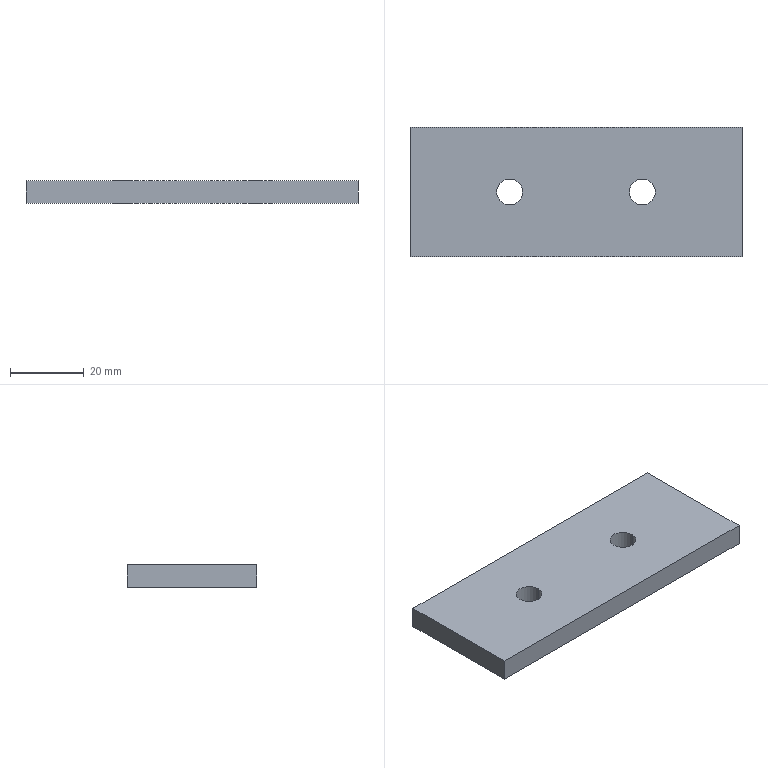Part | SolidWorks | features Extrusion 1, HoleWzd 1 | 1 solid | 10 faces | box 90 x 35 x 6 mm | volume 18438 mm3 | plane 6 | cylinder 4 | commonest cylinder face diameters 7 x4
STEP:
#1=CARTESIAN_POINT('',(23.5,17.5,0.));
#2=VERTEX_POINT('',#1);
#3=CARTESIAN_POINT('',(30.5,17.5,0.));
#4=VERTEX_POINT('',#3);
#5=CARTESIAN_POINT('',(27.,17.5,0.));
#6=DIRECTION('',(0.,0.,1.));
#7=DIRECTION('',(1.,0.,0.));
#8=AXIS2_PLACEMENT_3D('',#5,#6,#7);
#9=CIRCLE('',#8,3.5);
#10=EDGE_CURVE('',#2,#4,#9,.T.);
#11=ORIENTED_EDGE('',*,*,#10,.F.);
#12=CARTESIAN_POINT('',(23.5,17.5,6.));
#13=VERTEX_POINT('',#12);
#14=CARTESIAN_POINT('',(23.5,17.5,6.));
#15=DIRECTION('',(0.,0.,1.));
#16=VECTOR('',#15,1000.);
#17=LINE('',#14,#16);
#18=EDGE_CURVE('',#2,#13,#17,.T.);
#19=ORIENTED_EDGE('',*,*,#18,.T.);
#20=CARTESIAN_POINT('',(30.5,17.5,6.));
#21=VERTEX_POINT('',#20);
#22=CARTESIAN_POINT('',(27.,17.5,6.));
#23=DIRECTION('',(0.,0.,1.));
#24=DIRECTION('',(1.,0.,0.));
#25=AXIS2_PLACEMENT_3D('',#22,#23,#24);
#26=CIRCLE('',#25,3.5);
#27=EDGE_CURVE('',#13,#21,#26,.T.);
#28=ORIENTED_EDGE('',*,*,#27,.T.);
#29=CARTESIAN_POINT('',(30.5,17.5,6.));
#30=DIRECTION('',(0.,0.,1.));
#31=VECTOR('',#30,1000.);
#32=LINE('',#29,#31);
#33=EDGE_CURVE('',#4,#21,#32,.T.);
#34=ORIENTED_EDGE('',*,*,#33,.F.);
#35=EDGE_LOOP('',(#11,#19,#28,#34));
#36=FACE_OUTER_BOUND('',#35,.T.);
#37=CARTESIAN_POINT('',(27.,17.5,6.));
#38=DIRECTION('',(0.,0.,1.));
#39=DIRECTION('',(1.,0.,0.));
#40=AXIS2_PLACEMENT_3D('',#37,#38,#39);
#41=CYLINDRICAL_SURFACE('',#40,3.5);
#42=ADVANCED_FACE('',(#36),#41,.F.);
#43=CARTESIAN_POINT('',(59.5,17.5,0.));
#44=VERTEX_POINT('',#43);
#45=CARTESIAN_POINT('',(66.5,17.5,0.));
#46=VERTEX_POINT('',#45);
#47=CARTESIAN_POINT('',(63.,17.5,0.));
#48=DIRECTION('',(0.,0.,1.));
#49=DIRECTION('',(1.,0.,0.));
#50=AXIS2_PLACEMENT_3D('',#47,#48,#49);
#51=CIRCLE('',#50,3.5);
#52=EDGE_CURVE('',#44,#46,#51,.T.);
#53=ORIENTED_EDGE('',*,*,#52,.F.);
#54=CARTESIAN_POINT('',(59.5,17.5,6.));
#55=VERTEX_POINT('',#54);
#56=CARTESIAN_POINT('',(59.5,17.5,6.));
#57=DIRECTION('',(0.,0.,1.));
#58=VECTOR('',#57,1000.);
#59=LINE('',#56,#58);
#60=EDGE_CURVE('',#44,#55,#59,.T.);
#61=ORIENTED_EDGE('',*,*,#60,.T.);
#62=CARTESIAN_POINT('',(66.5,17.5,6.));
#63=VERTEX_POINT('',#62);
#64=CARTESIAN_POINT('',(63.,17.5,6.));
#65=DIRECTION('',(0.,0.,1.));
#66=DIRECTION('',(1.,0.,0.));
#67=AXIS2_PLACEMENT_3D('',#64,#65,#66);
#68=CIRCLE('',#67,3.5);
#69=EDGE_CURVE('',#55,#63,#68,.T.);
#70=ORIENTED_EDGE('',*,*,#69,.T.);
#71=CARTESIAN_POINT('',(66.5,17.5,6.));
#72=DIRECTION('',(0.,0.,1.));
#73=VECTOR('',#72,1000.);
#74=LINE('',#71,#73);
#75=EDGE_CURVE('',#46,#63,#74,.T.);
#76=ORIENTED_EDGE('',*,*,#75,.F.);
#77=EDGE_LOOP('',(#53,#61,#70,#76));
#78=FACE_OUTER_BOUND('',#77,.T.);
#79=CARTESIAN_POINT('',(63.,17.5,6.));
#80=DIRECTION('',(0.,0.,1.));
#81=DIRECTION('',(1.,0.,0.));
#82=AXIS2_PLACEMENT_3D('',#79,#80,#81);
#83=CYLINDRICAL_SURFACE('',#82,3.5);
#84=ADVANCED_FACE('',(#78),#83,.F.);
#85=CARTESIAN_POINT('',(0.,35.,0.));
#86=VERTEX_POINT('',#85);
#87=CARTESIAN_POINT('',(0.,0.,0.));
#88=VERTEX_POINT('',#87);
#89=CARTESIAN_POINT('',(0.,0.,0.));
#90=DIRECTION('',(0.,-1.,0.));
#91=VECTOR('',#90,1000.);
#92=LINE('',#89,#91);
#93=EDGE_CURVE('',#86,#88,#92,.T.);
#94=ORIENTED_EDGE('',*,*,#93,.T.);
#95=CARTESIAN_POINT('',(0.,0.,6.));
#96=VERTEX_POINT('',#95);
#97=CARTESIAN_POINT('',(0.,0.,6.));
#98=DIRECTION('',(0.,0.,-1.));
#99=VECTOR('',#98,1000.);
#100=LINE('',#97,#99);
#101=EDGE_CURVE('',#96,#88,#100,.T.);
#102=ORIENTED_EDGE('',*,*,#101,.F.);
#103=CARTESIAN_POINT('',(0.,35.,6.));
#104=VERTEX_POINT('',#103);
#105=CARTESIAN_POINT('',(0.,0.,6.));
#106=DIRECTION('',(0.,-1.,0.));
#107=VECTOR('',#106,1000.);
#108=LINE('',#105,#107);
#109=EDGE_CURVE('',#104,#96,#108,.T.);
#110=ORIENTED_EDGE('',*,*,#109,.F.);
#111=CARTESIAN_POINT('',(0.,35.,6.));
#112=DIRECTION('',(0.,0.,-1.));
#113=VECTOR('',#112,1000.);
#114=LINE('',#111,#113);
#115=EDGE_CURVE('',#104,#86,#114,.T.);
#116=ORIENTED_EDGE('',*,*,#115,.T.);
#117=EDGE_LOOP('',(#94,#102,#110,#116));
#118=FACE_OUTER_BOUND('',#117,.T.);
#119=CARTESIAN_POINT('',(0.,0.,6.));
#120=DIRECTION('',(1.,0.,0.));
#121=DIRECTION('',(0.,0.,-1.));
#122=AXIS2_PLACEMENT_3D('',#119,#120,#121);
#123=PLANE('',#122);
#124=ADVANCED_FACE('',(#118),#123,.F.);
#125=CARTESIAN_POINT('',(90.,0.,0.));
#126=VERTEX_POINT('',#125);
#127=CARTESIAN_POINT('',(0.,0.,0.));
#128=DIRECTION('',(1.,0.,0.));
#129=VECTOR('',#128,1000.);
#130=LINE('',#127,#129);
#131=EDGE_CURVE('',#88,#126,#130,.T.);
#132=ORIENTED_EDGE('',*,*,#131,.T.);
#133=CARTESIAN_POINT('',(90.,0.,6.));
#134=VERTEX_POINT('',#133);
#135=CARTESIAN_POINT('',(90.,0.,6.));
#136=DIRECTION('',(0.,0.,-1.));
#137=VECTOR('',#136,1000.);
#138=LINE('',#135,#137);
#139=EDGE_CURVE('',#134,#126,#138,.T.);
#140=ORIENTED_EDGE('',*,*,#139,.F.);
#141=CARTESIAN_POINT('',(0.,0.,6.));
#142=DIRECTION('',(1.,0.,0.));
#143=VECTOR('',#142,1000.);
#144=LINE('',#141,#143);
#145=EDGE_CURVE('',#96,#134,#144,.T.);
#146=ORIENTED_EDGE('',*,*,#145,.F.);
#147=ORIENTED_EDGE('',*,*,#101,.T.);
#148=EDGE_LOOP('',(#132,#140,#146,#147));
#149=FACE_OUTER_BOUND('',#148,.T.);
#150=CARTESIAN_POINT('',(0.,0.,6.));
#151=DIRECTION('',(0.,1.,0.));
#152=DIRECTION('',(0.,0.,1.));
#153=AXIS2_PLACEMENT_3D('',#150,#151,#152);
#154=PLANE('',#153);
#155=ADVANCED_FACE('',(#149),#154,.F.);
#156=CARTESIAN_POINT('',(90.,35.,0.));
#157=VERTEX_POINT('',#156);
#158=CARTESIAN_POINT('',(90.,0.,0.));
#159=DIRECTION('',(0.,1.,0.));
#160=VECTOR('',#159,1000.);
#161=LINE('',#158,#160);
#162=EDGE_CURVE('',#126,#157,#161,.T.);
#163=ORIENTED_EDGE('',*,*,#162,.T.);
#164=CARTESIAN_POINT('',(90.,35.,6.));
#165=VERTEX_POINT('',#164);
#166=CARTESIAN_POINT('',(90.,35.,6.));
#167=DIRECTION('',(0.,0.,-1.));
#168=VECTOR('',#167,1000.);
#169=LINE('',#166,#168);
#170=EDGE_CURVE('',#165,#157,#169,.T.);
#171=ORIENTED_EDGE('',*,*,#170,.F.);
#172=CARTESIAN_POINT('',(90.,0.,6.));
#173=DIRECTION('',(0.,1.,0.));
#174=VECTOR('',#173,1000.);
#175=LINE('',#172,#174);
#176=EDGE_CURVE('',#134,#165,#175,.T.);
#177=ORIENTED_EDGE('',*,*,#176,.F.);
#178=ORIENTED_EDGE('',*,*,#139,.T.);
#179=EDGE_LOOP('',(#163,#171,#177,#178));
#180=FACE_OUTER_BOUND('',#179,.T.);
#181=CARTESIAN_POINT('',(90.,0.,6.));
#182=DIRECTION('',(-1.,0.,0.));
#183=DIRECTION('',(0.,0.,1.));
#184=AXIS2_PLACEMENT_3D('',#181,#182,#183);
#185=PLANE('',#184);
#186=ADVANCED_FACE('',(#180),#185,.F.);
#187=CARTESIAN_POINT('',(0.,35.,0.));
#188=DIRECTION('',(-1.,0.,0.));
#189=VECTOR('',#188,1000.);
#190=LINE('',#187,#189);
#191=EDGE_CURVE('',#157,#86,#190,.T.);
#192=ORIENTED_EDGE('',*,*,#191,.T.);
#193=ORIENTED_EDGE('',*,*,#115,.F.);
#194=CARTESIAN_POINT('',(0.,35.,6.));
#195=DIRECTION('',(-1.,0.,0.));
#196=VECTOR('',#195,1000.);
#197=LINE('',#194,#196);
#198=EDGE_CURVE('',#165,#104,#197,.T.);
#199=ORIENTED_EDGE('',*,*,#198,.F.);
#200=ORIENTED_EDGE('',*,*,#170,.T.);
#201=EDGE_LOOP('',(#192,#193,#199,#200));
#202=FACE_OUTER_BOUND('',#201,.T.);
#203=CARTESIAN_POINT('',(0.,35.,6.));
#204=DIRECTION('',(0.,-1.,0.));
#205=DIRECTION('',(0.,0.,-1.));
#206=AXIS2_PLACEMENT_3D('',#203,#204,#205);
#207=PLANE('',#206);
#208=ADVANCED_FACE('',(#202),#207,.F.);
#209=CARTESIAN_POINT('',(27.,17.5,6.));
#210=DIRECTION('',(0.,0.,1.));
#211=DIRECTION('',(1.,0.,0.));
#212=AXIS2_PLACEMENT_3D('',#209,#210,#211);
#213=CIRCLE('',#212,3.5);
#214=EDGE_CURVE('',#21,#13,#213,.T.);
#215=ORIENTED_EDGE('',*,*,#214,.F.);
#216=ORIENTED_EDGE('',*,*,#27,.F.);
#217=EDGE_LOOP('',(#215,#216));
#218=FACE_BOUND('',#217,.T.);
#219=CARTESIAN_POINT('',(63.,17.5,6.));
#220=DIRECTION('',(0.,0.,1.));
#221=DIRECTION('',(1.,0.,0.));
#222=AXIS2_PLACEMENT_3D('',#219,#220,#221);
#223=CIRCLE('',#222,3.5);
#224=EDGE_CURVE('',#63,#55,#223,.T.);
#225=ORIENTED_EDGE('',*,*,#224,.F.);
#226=ORIENTED_EDGE('',*,*,#69,.F.);
#227=EDGE_LOOP('',(#225,#226));
#228=FACE_BOUND('',#227,.T.);
#229=ORIENTED_EDGE('',*,*,#109,.T.);
#230=ORIENTED_EDGE('',*,*,#145,.T.);
#231=ORIENTED_EDGE('',*,*,#176,.T.);
#232=ORIENTED_EDGE('',*,*,#198,.T.);
#233=EDGE_LOOP('',(#229,#230,#231,#232));
#234=FACE_OUTER_BOUND('',#233,.T.);
#235=CARTESIAN_POINT('',(0.,0.,6.));
#236=DIRECTION('',(0.,0.,-1.));
#237=DIRECTION('',(-1.,0.,0.));
#238=AXIS2_PLACEMENT_3D('',#235,#236,#237);
#239=PLANE('',#238);
#240=ADVANCED_FACE('',(#218,#228,#234),#239,.F.);
#241=CARTESIAN_POINT('',(27.,17.5,0.));
#242=DIRECTION('',(0.,0.,1.));
#243=DIRECTION('',(1.,0.,0.));
#244=AXIS2_PLACEMENT_3D('',#241,#242,#243);
#245=CIRCLE('',#244,3.5);
#246=EDGE_CURVE('',#4,#2,#245,.T.);
#247=ORIENTED_EDGE('',*,*,#246,.T.);
#248=ORIENTED_EDGE('',*,*,#10,.T.);
#249=EDGE_LOOP('',(#247,#248));
#250=FACE_BOUND('',#249,.T.);
#251=CARTESIAN_POINT('',(63.,17.5,0.));
#252=DIRECTION('',(0.,0.,1.));
#253=DIRECTION('',(1.,0.,0.));
#254=AXIS2_PLACEMENT_3D('',#251,#252,#253);
#255=CIRCLE('',#254,3.5);
#256=EDGE_CURVE('',#46,#44,#255,.T.);
#257=ORIENTED_EDGE('',*,*,#256,.T.);
#258=ORIENTED_EDGE('',*,*,#52,.T.);
#259=EDGE_LOOP('',(#257,#258));
#260=FACE_BOUND('',#259,.T.);
#261=ORIENTED_EDGE('',*,*,#93,.F.);
#262=ORIENTED_EDGE('',*,*,#191,.F.);
#263=ORIENTED_EDGE('',*,*,#162,.F.);
#264=ORIENTED_EDGE('',*,*,#131,.F.);
#265=EDGE_LOOP('',(#261,#262,#263,#264));
#266=FACE_OUTER_BOUND('',#265,.T.);
#267=CARTESIAN_POINT('',(0.,0.,0.));
#268=DIRECTION('',(0.,0.,-1.));
#269=DIRECTION('',(-1.,0.,0.));
#270=AXIS2_PLACEMENT_3D('',#267,#268,#269);
#271=PLANE('',#270);
#272=ADVANCED_FACE('',(#250,#260,#266),#271,.T.);
#273=ORIENTED_EDGE('',*,*,#60,.F.);
#274=ORIENTED_EDGE('',*,*,#256,.F.);
#275=ORIENTED_EDGE('',*,*,#75,.T.);
#276=ORIENTED_EDGE('',*,*,#224,.T.);
#277=EDGE_LOOP('',(#273,#274,#275,#276));
#278=FACE_OUTER_BOUND('',#277,.T.);
#279=CARTESIAN_POINT('',(63.,17.5,6.));
#280=DIRECTION('',(0.,0.,1.));
#281=DIRECTION('',(1.,0.,0.));
#282=AXIS2_PLACEMENT_3D('',#279,#280,#281);
#283=CYLINDRICAL_SURFACE('',#282,3.5);
#284=ADVANCED_FACE('',(#278),#283,.F.);
#285=ORIENTED_EDGE('',*,*,#18,.F.);
#286=ORIENTED_EDGE('',*,*,#246,.F.);
#287=ORIENTED_EDGE('',*,*,#33,.T.);
#288=ORIENTED_EDGE('',*,*,#214,.T.);
#289=EDGE_LOOP('',(#285,#286,#287,#288));
#290=FACE_OUTER_BOUND('',#289,.T.);
#291=CARTESIAN_POINT('',(27.,17.5,6.));
#292=DIRECTION('',(0.,0.,1.));
#293=DIRECTION('',(1.,0.,0.));
#294=AXIS2_PLACEMENT_3D('',#291,#292,#293);
#295=CYLINDRICAL_SURFACE('',#294,3.5);
#296=ADVANCED_FACE('',(#290),#295,.F.);
#297=CLOSED_SHELL('',(#42,#84,#124,#155,#186,#208,#240,#272,#284,#296));
#298=MANIFOLD_SOLID_BREP('',#297);
#299=CARTESIAN_POINT('',(0.,0.,0.));
#300=DIRECTION('',(0.,0.,1.));
#301=DIRECTION('',(1.,0.,0.));
#302=AXIS2_PLACEMENT_3D('',#299,#300,#301);
#303=(LENGTH_UNIT()NAMED_UNIT(*)SI_UNIT(.MILLI.,.METRE.));
#304=UNCERTAINTY_MEASURE_WITH_UNIT(LENGTH_MEASURE(0.00001),#303,'','');
#305=(NAMED_UNIT(*)PLANE_ANGLE_UNIT()SI_UNIT($,.RADIAN.));
#306=(NAMED_UNIT(*)SI_UNIT($,.STERADIAN.)SOLID_ANGLE_UNIT());
#307=(GEOMETRIC_REPRESENTATION_CONTEXT(3)GLOBAL_UNCERTAINTY_ASSIGNED_CONTEXT((#304))GLOBAL_UNIT_ASSIGNED_CONTEXT((#303,#305,#306))REPRESENTATION_CONTEXT('',''));
#308=ADVANCED_BREP_SHAPE_REPRESENTATION('',(#298,#302),#307);